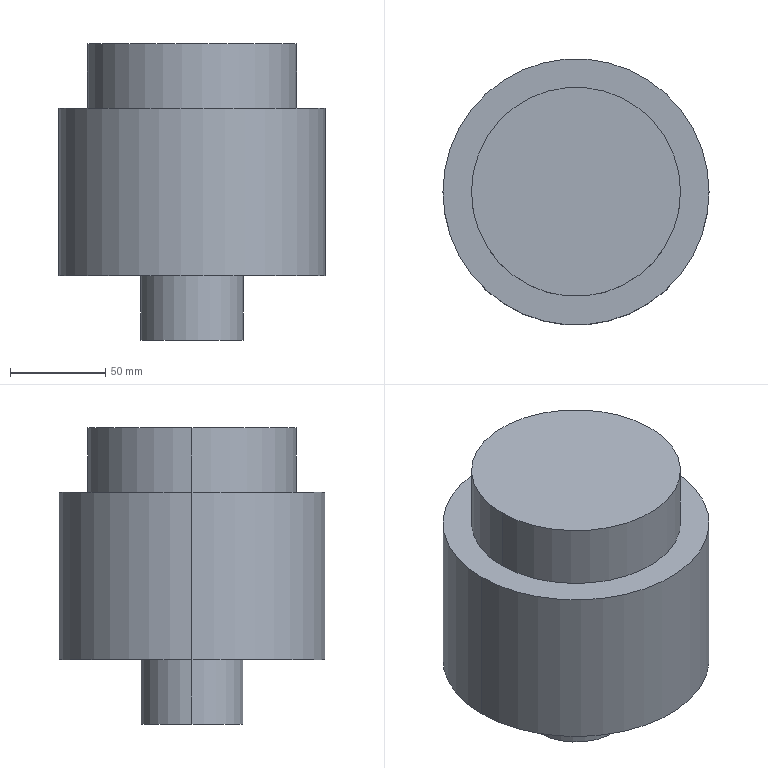Part | SolidWorks | features ICE 2, Extrusion 1 | 1 solid | 10 faces | box 140 x 140 x 156 mm | volume 1755635 mm3 | cylinder 6 | plane 4 | commonest cylinder face diameters 54 x2 110 x2 140 x2
STEP:
#1=CARTESIAN_POINT('',(55.,0.,156.));
#2=VERTEX_POINT('',#1);
#3=CARTESIAN_POINT('',(-55.,0.,156.));
#4=VERTEX_POINT('',#3);
#5=CARTESIAN_POINT('',(0.,0.,156.));
#6=DIRECTION('',(0.,0.,1.));
#7=DIRECTION('',(1.,0.,0.));
#8=AXIS2_PLACEMENT_3D('',#5,#6,#7);
#9=CIRCLE('',#8,55.);
#10=EDGE_CURVE('',#2,#4,#9,.T.);
#11=ORIENTED_EDGE('',*,*,#10,.F.);
#12=CARTESIAN_POINT('',(55.,0.,122.));
#13=VERTEX_POINT('',#12);
#14=CARTESIAN_POINT('',(55.,0.,156.));
#15=DIRECTION('',(0.,0.,-1.));
#16=VECTOR('',#15,1000.);
#17=LINE('',#14,#16);
#18=EDGE_CURVE('',#2,#13,#17,.T.);
#19=ORIENTED_EDGE('',*,*,#18,.T.);
#20=CARTESIAN_POINT('',(-55.,0.,122.));
#21=VERTEX_POINT('',#20);
#22=CARTESIAN_POINT('',(0.,0.,122.));
#23=DIRECTION('',(0.,0.,1.));
#24=DIRECTION('',(1.,0.,0.));
#25=AXIS2_PLACEMENT_3D('',#22,#23,#24);
#26=CIRCLE('',#25,55.);
#27=EDGE_CURVE('',#13,#21,#26,.T.);
#28=ORIENTED_EDGE('',*,*,#27,.T.);
#29=CARTESIAN_POINT('',(-55.,0.,156.));
#30=DIRECTION('',(0.,0.,-1.));
#31=VECTOR('',#30,1000.);
#32=LINE('',#29,#31);
#33=EDGE_CURVE('',#4,#21,#32,.T.);
#34=ORIENTED_EDGE('',*,*,#33,.F.);
#35=EDGE_LOOP('',(#11,#19,#28,#34));
#36=FACE_OUTER_BOUND('',#35,.T.);
#37=CARTESIAN_POINT('',(0.,0.,156.));
#38=DIRECTION('',(0.,0.,-1.));
#39=DIRECTION('',(-1.,0.,0.));
#40=AXIS2_PLACEMENT_3D('',#37,#38,#39);
#41=CYLINDRICAL_SURFACE('',#40,55.);
#42=ADVANCED_FACE('',(#36),#41,.T.);
#43=CARTESIAN_POINT('',(70.,0.,122.));
#44=VERTEX_POINT('',#43);
#45=CARTESIAN_POINT('',(-70.,0.,122.));
#46=VERTEX_POINT('',#45);
#47=CARTESIAN_POINT('',(0.,0.,122.));
#48=DIRECTION('',(0.,0.,1.));
#49=DIRECTION('',(1.,0.,0.));
#50=AXIS2_PLACEMENT_3D('',#47,#48,#49);
#51=CIRCLE('',#50,70.);
#52=EDGE_CURVE('',#44,#46,#51,.T.);
#53=ORIENTED_EDGE('',*,*,#52,.F.);
#54=CARTESIAN_POINT('',(70.,0.,34.));
#55=VERTEX_POINT('',#54);
#56=CARTESIAN_POINT('',(70.,0.,122.));
#57=DIRECTION('',(0.,0.,-1.));
#58=VECTOR('',#57,1000.);
#59=LINE('',#56,#58);
#60=EDGE_CURVE('',#44,#55,#59,.T.);
#61=ORIENTED_EDGE('',*,*,#60,.T.);
#62=CARTESIAN_POINT('',(-70.,0.,34.));
#63=VERTEX_POINT('',#62);
#64=CARTESIAN_POINT('',(0.,0.,34.));
#65=DIRECTION('',(0.,0.,1.));
#66=DIRECTION('',(1.,0.,0.));
#67=AXIS2_PLACEMENT_3D('',#64,#65,#66);
#68=CIRCLE('',#67,70.);
#69=EDGE_CURVE('',#55,#63,#68,.T.);
#70=ORIENTED_EDGE('',*,*,#69,.T.);
#71=CARTESIAN_POINT('',(-70.,0.,122.));
#72=DIRECTION('',(0.,0.,-1.));
#73=VECTOR('',#72,1000.);
#74=LINE('',#71,#73);
#75=EDGE_CURVE('',#46,#63,#74,.T.);
#76=ORIENTED_EDGE('',*,*,#75,.F.);
#77=EDGE_LOOP('',(#53,#61,#70,#76));
#78=FACE_OUTER_BOUND('',#77,.T.);
#79=CARTESIAN_POINT('',(0.,0.,122.));
#80=DIRECTION('',(0.,0.,-1.));
#81=DIRECTION('',(-1.,0.,0.));
#82=AXIS2_PLACEMENT_3D('',#79,#80,#81);
#83=CYLINDRICAL_SURFACE('',#82,70.);
#84=ADVANCED_FACE('',(#78),#83,.T.);
#85=CARTESIAN_POINT('',(27.,0.,34.));
#86=VERTEX_POINT('',#85);
#87=CARTESIAN_POINT('',(-27.,0.,34.));
#88=VERTEX_POINT('',#87);
#89=CARTESIAN_POINT('',(0.,0.,34.));
#90=DIRECTION('',(0.,0.,1.));
#91=DIRECTION('',(1.,0.,0.));
#92=AXIS2_PLACEMENT_3D('',#89,#90,#91);
#93=CIRCLE('',#92,27.);
#94=EDGE_CURVE('',#86,#88,#93,.T.);
#95=ORIENTED_EDGE('',*,*,#94,.F.);
#96=CARTESIAN_POINT('',(27.,0.,0.));
#97=VERTEX_POINT('',#96);
#98=CARTESIAN_POINT('',(27.,0.,34.));
#99=DIRECTION('',(0.,0.,-1.));
#100=VECTOR('',#99,1000.);
#101=LINE('',#98,#100);
#102=EDGE_CURVE('',#86,#97,#101,.T.);
#103=ORIENTED_EDGE('',*,*,#102,.T.);
#104=CARTESIAN_POINT('',(-27.,0.,0.));
#105=VERTEX_POINT('',#104);
#106=CARTESIAN_POINT('',(0.,0.,0.));
#107=DIRECTION('',(0.,0.,1.));
#108=DIRECTION('',(1.,0.,0.));
#109=AXIS2_PLACEMENT_3D('',#106,#107,#108);
#110=CIRCLE('',#109,27.);
#111=EDGE_CURVE('',#97,#105,#110,.T.);
#112=ORIENTED_EDGE('',*,*,#111,.T.);
#113=CARTESIAN_POINT('',(-27.,0.,34.));
#114=DIRECTION('',(0.,0.,-1.));
#115=VECTOR('',#114,1000.);
#116=LINE('',#113,#115);
#117=EDGE_CURVE('',#88,#105,#116,.T.);
#118=ORIENTED_EDGE('',*,*,#117,.F.);
#119=EDGE_LOOP('',(#95,#103,#112,#118));
#120=FACE_OUTER_BOUND('',#119,.T.);
#121=CARTESIAN_POINT('',(0.,0.,34.));
#122=DIRECTION('',(0.,0.,-1.));
#123=DIRECTION('',(-1.,0.,0.));
#124=AXIS2_PLACEMENT_3D('',#121,#122,#123);
#125=CYLINDRICAL_SURFACE('',#124,27.);
#126=ADVANCED_FACE('',(#120),#125,.T.);
#127=CARTESIAN_POINT('',(0.,0.,122.));
#128=DIRECTION('',(0.,0.,1.));
#129=DIRECTION('',(1.,0.,0.));
#130=AXIS2_PLACEMENT_3D('',#127,#128,#129);
#131=CIRCLE('',#130,70.);
#132=EDGE_CURVE('',#46,#44,#131,.T.);
#133=ORIENTED_EDGE('',*,*,#132,.T.);
#134=ORIENTED_EDGE('',*,*,#52,.T.);
#135=EDGE_LOOP('',(#133,#134));
#136=FACE_OUTER_BOUND('',#135,.T.);
#137=CARTESIAN_POINT('',(0.,0.,122.));
#138=DIRECTION('',(0.,0.,1.));
#139=DIRECTION('',(1.,0.,0.));
#140=AXIS2_PLACEMENT_3D('',#137,#138,#139);
#141=CIRCLE('',#140,55.);
#142=EDGE_CURVE('',#21,#13,#141,.T.);
#143=ORIENTED_EDGE('',*,*,#142,.F.);
#144=ORIENTED_EDGE('',*,*,#27,.F.);
#145=EDGE_LOOP('',(#143,#144));
#146=FACE_BOUND('',#145,.T.);
#147=CARTESIAN_POINT('',(0.,0.,122.));
#148=DIRECTION('',(0.,0.,1.));
#149=DIRECTION('',(1.,0.,0.));
#150=AXIS2_PLACEMENT_3D('',#147,#148,#149);
#151=PLANE('',#150);
#152=ADVANCED_FACE('',(#136,#146),#151,.T.);
#153=ORIENTED_EDGE('',*,*,#102,.F.);
#154=CARTESIAN_POINT('',(0.,0.,34.));
#155=DIRECTION('',(0.,0.,1.));
#156=DIRECTION('',(1.,0.,0.));
#157=AXIS2_PLACEMENT_3D('',#154,#155,#156);
#158=CIRCLE('',#157,27.);
#159=EDGE_CURVE('',#88,#86,#158,.T.);
#160=ORIENTED_EDGE('',*,*,#159,.F.);
#161=ORIENTED_EDGE('',*,*,#117,.T.);
#162=CARTESIAN_POINT('',(0.,0.,0.));
#163=DIRECTION('',(0.,0.,1.));
#164=DIRECTION('',(1.,0.,0.));
#165=AXIS2_PLACEMENT_3D('',#162,#163,#164);
#166=CIRCLE('',#165,27.);
#167=EDGE_CURVE('',#105,#97,#166,.T.);
#168=ORIENTED_EDGE('',*,*,#167,.T.);
#169=EDGE_LOOP('',(#153,#160,#161,#168));
#170=FACE_OUTER_BOUND('',#169,.T.);
#171=CARTESIAN_POINT('',(0.,0.,34.));
#172=DIRECTION('',(0.,0.,-1.));
#173=DIRECTION('',(-1.,0.,0.));
#174=AXIS2_PLACEMENT_3D('',#171,#172,#173);
#175=CYLINDRICAL_SURFACE('',#174,27.);
#176=ADVANCED_FACE('',(#170),#175,.T.);
#177=ORIENTED_EDGE('',*,*,#167,.F.);
#178=ORIENTED_EDGE('',*,*,#111,.F.);
#179=EDGE_LOOP('',(#177,#178));
#180=FACE_OUTER_BOUND('',#179,.T.);
#181=CARTESIAN_POINT('',(0.,0.,0.));
#182=DIRECTION('',(0.,0.,1.));
#183=DIRECTION('',(1.,0.,0.));
#184=AXIS2_PLACEMENT_3D('',#181,#182,#183);
#185=PLANE('',#184);
#186=ADVANCED_FACE('',(#180),#185,.F.);
#187=CARTESIAN_POINT('',(0.,0.,34.));
#188=DIRECTION('',(0.,0.,1.));
#189=DIRECTION('',(1.,0.,0.));
#190=AXIS2_PLACEMENT_3D('',#187,#188,#189);
#191=CIRCLE('',#190,70.);
#192=EDGE_CURVE('',#63,#55,#191,.T.);
#193=ORIENTED_EDGE('',*,*,#192,.F.);
#194=ORIENTED_EDGE('',*,*,#69,.F.);
#195=EDGE_LOOP('',(#193,#194));
#196=FACE_OUTER_BOUND('',#195,.T.);
#197=ORIENTED_EDGE('',*,*,#159,.T.);
#198=ORIENTED_EDGE('',*,*,#94,.T.);
#199=EDGE_LOOP('',(#197,#198));
#200=FACE_BOUND('',#199,.T.);
#201=CARTESIAN_POINT('',(0.,0.,34.));
#202=DIRECTION('',(0.,0.,1.));
#203=DIRECTION('',(1.,0.,0.));
#204=AXIS2_PLACEMENT_3D('',#201,#202,#203);
#205=PLANE('',#204);
#206=ADVANCED_FACE('',(#196,#200),#205,.F.);
#207=ORIENTED_EDGE('',*,*,#60,.F.);
#208=ORIENTED_EDGE('',*,*,#132,.F.);
#209=ORIENTED_EDGE('',*,*,#75,.T.);
#210=ORIENTED_EDGE('',*,*,#192,.T.);
#211=EDGE_LOOP('',(#207,#208,#209,#210));
#212=FACE_OUTER_BOUND('',#211,.T.);
#213=CARTESIAN_POINT('',(0.,0.,122.));
#214=DIRECTION('',(0.,0.,-1.));
#215=DIRECTION('',(-1.,0.,0.));
#216=AXIS2_PLACEMENT_3D('',#213,#214,#215);
#217=CYLINDRICAL_SURFACE('',#216,70.);
#218=ADVANCED_FACE('',(#212),#217,.T.);
#219=ORIENTED_EDGE('',*,*,#18,.F.);
#220=CARTESIAN_POINT('',(0.,0.,156.));
#221=DIRECTION('',(0.,0.,1.));
#222=DIRECTION('',(1.,0.,0.));
#223=AXIS2_PLACEMENT_3D('',#220,#221,#222);
#224=CIRCLE('',#223,55.);
#225=EDGE_CURVE('',#4,#2,#224,.T.);
#226=ORIENTED_EDGE('',*,*,#225,.F.);
#227=ORIENTED_EDGE('',*,*,#33,.T.);
#228=ORIENTED_EDGE('',*,*,#142,.T.);
#229=EDGE_LOOP('',(#219,#226,#227,#228));
#230=FACE_OUTER_BOUND('',#229,.T.);
#231=CARTESIAN_POINT('',(0.,0.,156.));
#232=DIRECTION('',(0.,0.,-1.));
#233=DIRECTION('',(-1.,0.,0.));
#234=AXIS2_PLACEMENT_3D('',#231,#232,#233);
#235=CYLINDRICAL_SURFACE('',#234,55.);
#236=ADVANCED_FACE('',(#230),#235,.T.);
#237=ORIENTED_EDGE('',*,*,#225,.T.);
#238=ORIENTED_EDGE('',*,*,#10,.T.);
#239=EDGE_LOOP('',(#237,#238));
#240=FACE_OUTER_BOUND('',#239,.T.);
#241=CARTESIAN_POINT('',(0.,0.,156.));
#242=DIRECTION('',(0.,0.,1.));
#243=DIRECTION('',(1.,0.,0.));
#244=AXIS2_PLACEMENT_3D('',#241,#242,#243);
#245=PLANE('',#244);
#246=ADVANCED_FACE('',(#240),#245,.T.);
#247=CLOSED_SHELL('',(#42,#84,#126,#152,#176,#186,#206,#218,#236,#246));
#248=MANIFOLD_SOLID_BREP('',#247);
#249=CARTESIAN_POINT('',(0.,0.,0.));
#250=DIRECTION('',(0.,0.,1.));
#251=DIRECTION('',(1.,0.,0.));
#252=AXIS2_PLACEMENT_3D('',#249,#250,#251);
#253=(LENGTH_UNIT()NAMED_UNIT(*)SI_UNIT(.MILLI.,.METRE.));
#254=UNCERTAINTY_MEASURE_WITH_UNIT(LENGTH_MEASURE(0.00001),#253,'','');
#255=(NAMED_UNIT(*)PLANE_ANGLE_UNIT()SI_UNIT($,.RADIAN.));
#256=(NAMED_UNIT(*)SI_UNIT($,.STERADIAN.)SOLID_ANGLE_UNIT());
#257=(GEOMETRIC_REPRESENTATION_CONTEXT(3)GLOBAL_UNCERTAINTY_ASSIGNED_CONTEXT((#254))GLOBAL_UNIT_ASSIGNED_CONTEXT((#253,#255,#256))REPRESENTATION_CONTEXT('',''));
#258=ADVANCED_BREP_SHAPE_REPRESENTATION('',(#248,#252),#257);